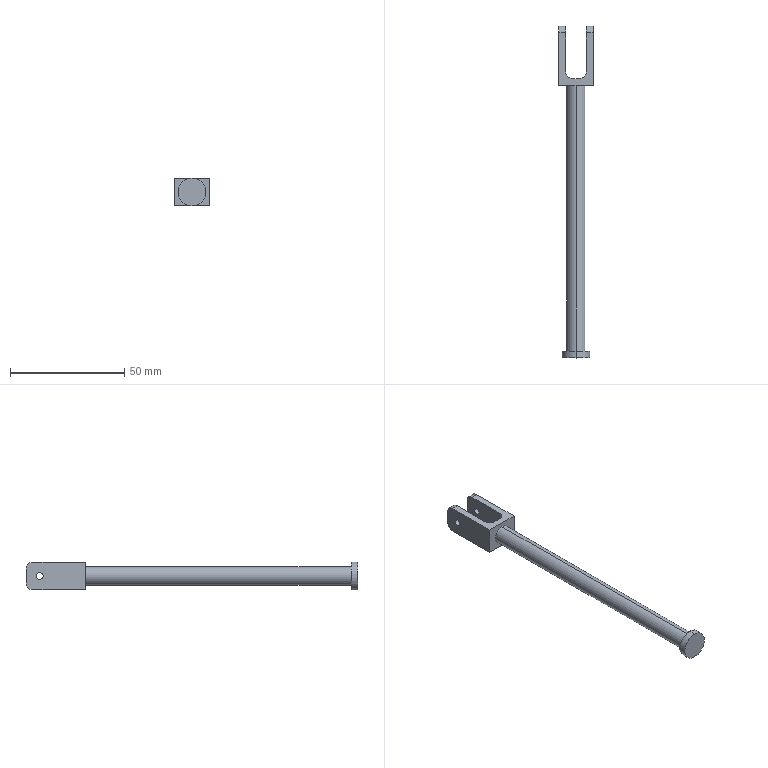Part | SolidWorks | features ICE 3, Fillet 2, Extrusion 1 | 1 solid | 26 faces | box 15 x 145 x 12.163 mm | volume 8356 mm3 | cylinder 14 | plane 12 | commonest cylinder face diameters 6 x6 3 x4 8 x2 12.163 x2
STEP:
#1=CARTESIAN_POINT('',(7.5,-119.,-0.08166));
#2=VERTEX_POINT('',#1);
#3=CARTESIAN_POINT('',(7.5,-119.,12.082));
#4=VERTEX_POINT('',#3);
#5=CARTESIAN_POINT('',(7.5,-119.,6.));
#6=DIRECTION('',(0.,-1.,0.));
#7=DIRECTION('',(0.,0.,-1.));
#8=AXIS2_PLACEMENT_3D('',#5,#6,#7);
#9=CIRCLE('',#8,6.082);
#10=EDGE_CURVE('',#2,#4,#9,.T.);
#11=ORIENTED_EDGE('',*,*,#10,.F.);
#12=CARTESIAN_POINT('',(7.5,-116.,-0.08166));
#13=VERTEX_POINT('',#12);
#14=CARTESIAN_POINT('',(7.5,-119.,-0.08166));
#15=DIRECTION('',(0.,1.,0.));
#16=VECTOR('',#15,1000.);
#17=LINE('',#14,#16);
#18=EDGE_CURVE('',#2,#13,#17,.T.);
#19=ORIENTED_EDGE('',*,*,#18,.T.);
#20=CARTESIAN_POINT('',(7.5,-116.,12.082));
#21=VERTEX_POINT('',#20);
#22=CARTESIAN_POINT('',(7.5,-116.,6.));
#23=DIRECTION('',(0.,-1.,0.));
#24=DIRECTION('',(0.,0.,-1.));
#25=AXIS2_PLACEMENT_3D('',#22,#23,#24);
#26=CIRCLE('',#25,6.082);
#27=EDGE_CURVE('',#13,#21,#26,.T.);
#28=ORIENTED_EDGE('',*,*,#27,.T.);
#29=CARTESIAN_POINT('',(7.5,-119.,12.082));
#30=DIRECTION('',(0.,1.,0.));
#31=VECTOR('',#30,1000.);
#32=LINE('',#29,#31);
#33=EDGE_CURVE('',#4,#21,#32,.T.);
#34=ORIENTED_EDGE('',*,*,#33,.F.);
#35=EDGE_LOOP('',(#11,#19,#28,#34));
#36=FACE_OUTER_BOUND('',#35,.T.);
#37=CARTESIAN_POINT('',(7.5,-119.,6.));
#38=DIRECTION('',(0.,1.,0.));
#39=DIRECTION('',(0.,0.,1.));
#40=AXIS2_PLACEMENT_3D('',#37,#38,#39);
#41=CYLINDRICAL_SURFACE('',#40,6.082);
#42=ADVANCED_FACE('',(#36),#41,.T.);
#43=CARTESIAN_POINT('',(7.5,-116.,2.));
#44=VERTEX_POINT('',#43);
#45=CARTESIAN_POINT('',(7.5,-116.,10.));
#46=VERTEX_POINT('',#45);
#47=CARTESIAN_POINT('',(7.5,-116.,6.));
#48=DIRECTION('',(0.,-1.,0.));
#49=DIRECTION('',(0.,0.,-1.));
#50=AXIS2_PLACEMENT_3D('',#47,#48,#49);
#51=CIRCLE('',#50,4.);
#52=EDGE_CURVE('',#44,#46,#51,.T.);
#53=ORIENTED_EDGE('',*,*,#52,.F.);
#54=CARTESIAN_POINT('',(7.5,0.,2.));
#55=VERTEX_POINT('',#54);
#56=CARTESIAN_POINT('',(7.5,-116.,2.));
#57=DIRECTION('',(0.,1.,0.));
#58=VECTOR('',#57,1000.);
#59=LINE('',#56,#58);
#60=EDGE_CURVE('',#44,#55,#59,.T.);
#61=ORIENTED_EDGE('',*,*,#60,.T.);
#62=CARTESIAN_POINT('',(7.5,0.,10.));
#63=VERTEX_POINT('',#62);
#64=CARTESIAN_POINT('',(7.5,0.,6.));
#65=DIRECTION('',(0.,-1.,0.));
#66=DIRECTION('',(0.,0.,-1.));
#67=AXIS2_PLACEMENT_3D('',#64,#65,#66);
#68=CIRCLE('',#67,4.);
#69=EDGE_CURVE('',#55,#63,#68,.T.);
#70=ORIENTED_EDGE('',*,*,#69,.T.);
#71=CARTESIAN_POINT('',(7.5,-116.,10.));
#72=DIRECTION('',(0.,1.,0.));
#73=VECTOR('',#72,1000.);
#74=LINE('',#71,#73);
#75=EDGE_CURVE('',#46,#63,#74,.T.);
#76=ORIENTED_EDGE('',*,*,#75,.F.);
#77=EDGE_LOOP('',(#53,#61,#70,#76));
#78=FACE_OUTER_BOUND('',#77,.T.);
#79=CARTESIAN_POINT('',(7.5,-116.,6.));
#80=DIRECTION('',(0.,1.,0.));
#81=DIRECTION('',(0.,0.,1.));
#82=AXIS2_PLACEMENT_3D('',#79,#80,#81);
#83=CYLINDRICAL_SURFACE('',#82,4.);
#84=ADVANCED_FACE('',(#78),#83,.T.);
#85=CARTESIAN_POINT('',(12.,18.5,6.));
#86=VERTEX_POINT('',#85);
#87=CARTESIAN_POINT('',(12.,21.5,6.));
#88=VERTEX_POINT('',#87);
#89=CARTESIAN_POINT('',(12.,20.,6.));
#90=DIRECTION('',(1.,0.,0.));
#91=DIRECTION('',(0.,0.,-1.));
#92=AXIS2_PLACEMENT_3D('',#89,#90,#91);
#93=CIRCLE('',#92,1.5);
#94=EDGE_CURVE('',#86,#88,#93,.T.);
#95=ORIENTED_EDGE('',*,*,#94,.F.);
#96=CARTESIAN_POINT('',(15.,18.5,6.));
#97=VERTEX_POINT('',#96);
#98=CARTESIAN_POINT('',(0.,18.5,6.));
#99=DIRECTION('',(1.,0.,0.));
#100=VECTOR('',#99,1000.);
#101=LINE('',#98,#100);
#102=EDGE_CURVE('',#86,#97,#101,.T.);
#103=ORIENTED_EDGE('',*,*,#102,.T.);
#104=CARTESIAN_POINT('',(15.,21.5,6.));
#105=VERTEX_POINT('',#104);
#106=CARTESIAN_POINT('',(15.,20.,6.));
#107=DIRECTION('',(1.,0.,0.));
#108=DIRECTION('',(0.,1.,0.));
#109=AXIS2_PLACEMENT_3D('',#106,#107,#108);
#110=CIRCLE('',#109,1.5);
#111=EDGE_CURVE('',#97,#105,#110,.T.);
#112=ORIENTED_EDGE('',*,*,#111,.T.);
#113=CARTESIAN_POINT('',(0.,21.5,6.));
#114=DIRECTION('',(1.,0.,0.));
#115=VECTOR('',#114,1000.);
#116=LINE('',#113,#115);
#117=EDGE_CURVE('',#88,#105,#116,.T.);
#118=ORIENTED_EDGE('',*,*,#117,.F.);
#119=EDGE_LOOP('',(#95,#103,#112,#118));
#120=FACE_OUTER_BOUND('',#119,.T.);
#121=CARTESIAN_POINT('',(0.,20.,6.));
#122=DIRECTION('',(1.,0.,0.));
#123=DIRECTION('',(0.,1.,0.));
#124=AXIS2_PLACEMENT_3D('',#121,#122,#123);
#125=CYLINDRICAL_SURFACE('',#124,1.5);
#126=ADVANCED_FACE('',(#120),#125,.F.);
#127=CARTESIAN_POINT('',(0.,18.5,6.));
#128=VERTEX_POINT('',#127);
#129=CARTESIAN_POINT('',(0.,21.5,6.));
#130=VERTEX_POINT('',#129);
#131=CARTESIAN_POINT('',(0.,20.,6.));
#132=DIRECTION('',(1.,0.,0.));
#133=DIRECTION('',(0.,1.,0.));
#134=AXIS2_PLACEMENT_3D('',#131,#132,#133);
#135=CIRCLE('',#134,1.5);
#136=EDGE_CURVE('',#128,#130,#135,.T.);
#137=ORIENTED_EDGE('',*,*,#136,.F.);
#138=CARTESIAN_POINT('',(3.,18.5,6.));
#139=VERTEX_POINT('',#138);
#140=CARTESIAN_POINT('',(0.,18.5,6.));
#141=DIRECTION('',(1.,0.,0.));
#142=VECTOR('',#141,1000.);
#143=LINE('',#140,#142);
#144=EDGE_CURVE('',#128,#139,#143,.T.);
#145=ORIENTED_EDGE('',*,*,#144,.T.);
#146=CARTESIAN_POINT('',(3.,21.5,6.));
#147=VERTEX_POINT('',#146);
#148=CARTESIAN_POINT('',(3.,20.,6.));
#149=DIRECTION('',(-1.,0.,0.));
#150=DIRECTION('',(0.,0.,1.));
#151=AXIS2_PLACEMENT_3D('',#148,#149,#150);
#152=CIRCLE('',#151,1.5);
#153=EDGE_CURVE('',#147,#139,#152,.T.);
#154=ORIENTED_EDGE('',*,*,#153,.F.);
#155=CARTESIAN_POINT('',(0.,21.5,6.));
#156=DIRECTION('',(1.,0.,0.));
#157=VECTOR('',#156,1000.);
#158=LINE('',#155,#157);
#159=EDGE_CURVE('',#130,#147,#158,.T.);
#160=ORIENTED_EDGE('',*,*,#159,.F.);
#161=EDGE_LOOP('',(#137,#145,#154,#160));
#162=FACE_OUTER_BOUND('',#161,.T.);
#163=CARTESIAN_POINT('',(0.,20.,6.));
#164=DIRECTION('',(1.,0.,0.));
#165=DIRECTION('',(0.,1.,0.));
#166=AXIS2_PLACEMENT_3D('',#163,#164,#165);
#167=CYLINDRICAL_SURFACE('',#166,1.5);
#168=ADVANCED_FACE('',(#162),#167,.F.);
#169=CARTESIAN_POINT('',(3.,26.,9.));
#170=VERTEX_POINT('',#169);
#171=CARTESIAN_POINT('',(3.,26.,3.));
#172=VERTEX_POINT('',#171);
#173=CARTESIAN_POINT('',(3.,26.,12.));
#174=DIRECTION('',(0.,0.,-1.));
#175=VECTOR('',#174,1000.);
#176=LINE('',#173,#175);
#177=EDGE_CURVE('',#170,#172,#176,.T.);
#178=ORIENTED_EDGE('',*,*,#177,.T.);
#179=CARTESIAN_POINT('',(0.,26.,3.));
#180=VERTEX_POINT('',#179);
#181=CARTESIAN_POINT('',(3.,26.,3.));
#182=DIRECTION('',(-1.,0.,0.));
#183=VECTOR('',#182,1000.);
#184=LINE('',#181,#183);
#185=EDGE_CURVE('',#172,#180,#184,.T.);
#186=ORIENTED_EDGE('',*,*,#185,.T.);
#187=CARTESIAN_POINT('',(0.,26.,9.));
#188=VERTEX_POINT('',#187);
#189=CARTESIAN_POINT('',(0.,26.,12.));
#190=DIRECTION('',(0.,0.,-1.));
#191=VECTOR('',#190,1000.);
#192=LINE('',#189,#191);
#193=EDGE_CURVE('',#188,#180,#192,.T.);
#194=ORIENTED_EDGE('',*,*,#193,.F.);
#195=CARTESIAN_POINT('',(3.,26.,9.));
#196=DIRECTION('',(1.,0.,0.));
#197=VECTOR('',#196,1000.);
#198=LINE('',#195,#197);
#199=EDGE_CURVE('',#188,#170,#198,.T.);
#200=ORIENTED_EDGE('',*,*,#199,.T.);
#201=EDGE_LOOP('',(#178,#186,#194,#200));
#202=FACE_OUTER_BOUND('',#201,.T.);
#203=CARTESIAN_POINT('',(3.,26.,12.));
#204=DIRECTION('',(0.,-1.,0.));
#205=DIRECTION('',(0.,0.,-1.));
#206=AXIS2_PLACEMENT_3D('',#203,#204,#205);
#207=PLANE('',#206);
#208=ADVANCED_FACE('',(#202),#207,.F.);
#209=CARTESIAN_POINT('',(0.,20.,6.));
#210=DIRECTION('',(1.,0.,0.));
#211=DIRECTION('',(0.,1.,0.));
#212=AXIS2_PLACEMENT_3D('',#209,#210,#211);
#213=CIRCLE('',#212,1.5);
#214=EDGE_CURVE('',#130,#128,#213,.T.);
#215=ORIENTED_EDGE('',*,*,#214,.T.);
#216=ORIENTED_EDGE('',*,*,#136,.T.);
#217=EDGE_LOOP('',(#215,#216));
#218=FACE_BOUND('',#217,.T.);
#219=ORIENTED_EDGE('',*,*,#193,.T.);
#220=CARTESIAN_POINT('',(0.,23.,0.));
#221=VERTEX_POINT('',#220);
#222=CARTESIAN_POINT('',(0.,23.,3.));
#223=DIRECTION('',(-1.,0.,0.));
#224=DIRECTION('',(0.,1.,0.));
#225=AXIS2_PLACEMENT_3D('',#222,#223,#224);
#226=CIRCLE('',#225,3.);
#227=EDGE_CURVE('',#180,#221,#226,.T.);
#228=ORIENTED_EDGE('',*,*,#227,.T.);
#229=CARTESIAN_POINT('',(0.,0.,0.));
#230=VERTEX_POINT('',#229);
#231=CARTESIAN_POINT('',(0.,26.,0.));
#232=DIRECTION('',(0.,-1.,0.));
#233=VECTOR('',#232,1000.);
#234=LINE('',#231,#233);
#235=EDGE_CURVE('',#221,#230,#234,.T.);
#236=ORIENTED_EDGE('',*,*,#235,.T.);
#237=CARTESIAN_POINT('',(0.,0.,12.));
#238=VERTEX_POINT('',#237);
#239=CARTESIAN_POINT('',(0.,0.,12.));
#240=DIRECTION('',(0.,0.,-1.));
#241=VECTOR('',#240,1000.);
#242=LINE('',#239,#241);
#243=EDGE_CURVE('',#238,#230,#242,.T.);
#244=ORIENTED_EDGE('',*,*,#243,.F.);
#245=CARTESIAN_POINT('',(0.,23.,12.));
#246=VERTEX_POINT('',#245);
#247=CARTESIAN_POINT('',(0.,26.,12.));
#248=DIRECTION('',(0.,-1.,0.));
#249=VECTOR('',#248,1000.);
#250=LINE('',#247,#249);
#251=EDGE_CURVE('',#246,#238,#250,.T.);
#252=ORIENTED_EDGE('',*,*,#251,.F.);
#253=CARTESIAN_POINT('',(0.,23.,9.));
#254=DIRECTION('',(-1.,0.,0.));
#255=DIRECTION('',(0.,1.,0.));
#256=AXIS2_PLACEMENT_3D('',#253,#254,#255);
#257=CIRCLE('',#256,3.);
#258=EDGE_CURVE('',#246,#188,#257,.T.);
#259=ORIENTED_EDGE('',*,*,#258,.T.);
#260=EDGE_LOOP('',(#219,#228,#236,#244,#252,#259));
#261=FACE_OUTER_BOUND('',#260,.T.);
#262=CARTESIAN_POINT('',(0.,26.,12.));
#263=DIRECTION('',(1.,0.,0.));
#264=DIRECTION('',(0.,1.,0.));
#265=AXIS2_PLACEMENT_3D('',#262,#263,#264);
#266=PLANE('',#265);
#267=ADVANCED_FACE('',(#218,#261),#266,.F.);
#268=CARTESIAN_POINT('',(7.5,0.,6.));
#269=DIRECTION('',(0.,-1.,0.));
#270=DIRECTION('',(0.,0.,-1.));
#271=AXIS2_PLACEMENT_3D('',#268,#269,#270);
#272=CIRCLE('',#271,4.);
#273=EDGE_CURVE('',#63,#55,#272,.T.);
#274=ORIENTED_EDGE('',*,*,#273,.F.);
#275=ORIENTED_EDGE('',*,*,#69,.F.);
#276=EDGE_LOOP('',(#274,#275));
#277=FACE_BOUND('',#276,.T.);
#278=CARTESIAN_POINT('',(15.,0.,0.));
#279=VERTEX_POINT('',#278);
#280=CARTESIAN_POINT('',(0.,0.,0.));
#281=DIRECTION('',(1.,0.,0.));
#282=VECTOR('',#281,1000.);
#283=LINE('',#280,#282);
#284=EDGE_CURVE('',#230,#279,#283,.T.);
#285=ORIENTED_EDGE('',*,*,#284,.T.);
#286=CARTESIAN_POINT('',(15.,0.,12.));
#287=VERTEX_POINT('',#286);
#288=CARTESIAN_POINT('',(15.,0.,12.));
#289=DIRECTION('',(0.,0.,-1.));
#290=VECTOR('',#289,1000.);
#291=LINE('',#288,#290);
#292=EDGE_CURVE('',#287,#279,#291,.T.);
#293=ORIENTED_EDGE('',*,*,#292,.F.);
#294=CARTESIAN_POINT('',(0.,0.,12.));
#295=DIRECTION('',(1.,0.,0.));
#296=VECTOR('',#295,1000.);
#297=LINE('',#294,#296);
#298=EDGE_CURVE('',#238,#287,#297,.T.);
#299=ORIENTED_EDGE('',*,*,#298,.F.);
#300=ORIENTED_EDGE('',*,*,#243,.T.);
#301=EDGE_LOOP('',(#285,#293,#299,#300));
#302=FACE_OUTER_BOUND('',#301,.T.);
#303=CARTESIAN_POINT('',(0.,0.,12.));
#304=DIRECTION('',(0.,1.,0.));
#305=DIRECTION('',(0.,0.,1.));
#306=AXIS2_PLACEMENT_3D('',#303,#304,#305);
#307=PLANE('',#306);
#308=ADVANCED_FACE('',(#277,#302),#307,.F.);
#309=CARTESIAN_POINT('',(15.,20.,6.));
#310=DIRECTION('',(1.,0.,0.));
#311=DIRECTION('',(0.,1.,0.));
#312=AXIS2_PLACEMENT_3D('',#309,#310,#311);
#313=CIRCLE('',#312,1.5);
#314=EDGE_CURVE('',#105,#97,#313,.T.);
#315=ORIENTED_EDGE('',*,*,#314,.F.);
#316=ORIENTED_EDGE('',*,*,#111,.F.);
#317=EDGE_LOOP('',(#315,#316));
#318=FACE_BOUND('',#317,.T.);
#319=CARTESIAN_POINT('',(15.,23.,0.));
#320=VERTEX_POINT('',#319);
#321=CARTESIAN_POINT('',(15.,0.,0.));
#322=DIRECTION('',(0.,1.,0.));
#323=VECTOR('',#322,1000.);
#324=LINE('',#321,#323);
#325=EDGE_CURVE('',#279,#320,#324,.T.);
#326=ORIENTED_EDGE('',*,*,#325,.T.);
#327=CARTESIAN_POINT('',(15.,26.,3.));
#328=VERTEX_POINT('',#327);
#329=CARTESIAN_POINT('',(15.,23.,3.));
#330=DIRECTION('',(1.,0.,0.));
#331=DIRECTION('',(0.,-1.,0.));
#332=AXIS2_PLACEMENT_3D('',#329,#330,#331);
#333=CIRCLE('',#332,3.);
#334=EDGE_CURVE('',#320,#328,#333,.T.);
#335=ORIENTED_EDGE('',*,*,#334,.T.);
#336=CARTESIAN_POINT('',(15.,26.,9.));
#337=VERTEX_POINT('',#336);
#338=CARTESIAN_POINT('',(15.,26.,12.));
#339=DIRECTION('',(0.,0.,-1.));
#340=VECTOR('',#339,1000.);
#341=LINE('',#338,#340);
#342=EDGE_CURVE('',#337,#328,#341,.T.);
#343=ORIENTED_EDGE('',*,*,#342,.F.);
#344=CARTESIAN_POINT('',(15.,23.,12.));
#345=VERTEX_POINT('',#344);
#346=CARTESIAN_POINT('',(15.,23.,9.));
#347=DIRECTION('',(1.,0.,0.));
#348=DIRECTION('',(0.,-1.,0.));
#349=AXIS2_PLACEMENT_3D('',#346,#347,#348);
#350=CIRCLE('',#349,3.);
#351=EDGE_CURVE('',#337,#345,#350,.T.);
#352=ORIENTED_EDGE('',*,*,#351,.T.);
#353=CARTESIAN_POINT('',(15.,0.,12.));
#354=DIRECTION('',(0.,1.,0.));
#355=VECTOR('',#354,1000.);
#356=LINE('',#353,#355);
#357=EDGE_CURVE('',#287,#345,#356,.T.);
#358=ORIENTED_EDGE('',*,*,#357,.F.);
#359=ORIENTED_EDGE('',*,*,#292,.T.);
#360=EDGE_LOOP('',(#326,#335,#343,#352,#358,#359));
#361=FACE_OUTER_BOUND('',#360,.T.);
#362=CARTESIAN_POINT('',(15.,0.,12.));
#363=DIRECTION('',(-1.,0.,0.));
#364=DIRECTION('',(0.,-1.,0.));
#365=AXIS2_PLACEMENT_3D('',#362,#363,#364);
#366=PLANE('',#365);
#367=ADVANCED_FACE('',(#318,#361),#366,.F.);
#368=ORIENTED_EDGE('',*,*,#342,.T.);
#369=CARTESIAN_POINT('',(12.,26.,3.));
#370=VERTEX_POINT('',#369);
#371=CARTESIAN_POINT('',(15.,26.,3.));
#372=DIRECTION('',(-1.,0.,0.));
#373=VECTOR('',#372,1000.);
#374=LINE('',#371,#373);
#375=EDGE_CURVE('',#328,#370,#374,.T.);
#376=ORIENTED_EDGE('',*,*,#375,.T.);
#377=CARTESIAN_POINT('',(12.,26.,9.));
#378=VERTEX_POINT('',#377);
#379=CARTESIAN_POINT('',(12.,26.,12.));
#380=DIRECTION('',(0.,0.,-1.));
#381=VECTOR('',#380,1000.);
#382=LINE('',#379,#381);
#383=EDGE_CURVE('',#378,#370,#382,.T.);
#384=ORIENTED_EDGE('',*,*,#383,.F.);
#385=CARTESIAN_POINT('',(15.,26.,9.));
#386=DIRECTION('',(1.,0.,0.));
#387=VECTOR('',#386,1000.);
#388=LINE('',#385,#387);
#389=EDGE_CURVE('',#378,#337,#388,.T.);
#390=ORIENTED_EDGE('',*,*,#389,.T.);
#391=EDGE_LOOP('',(#368,#376,#384,#390));
#392=FACE_OUTER_BOUND('',#391,.T.);
#393=CARTESIAN_POINT('',(15.,26.,12.));
#394=DIRECTION('',(0.,-1.,0.));
#395=DIRECTION('',(0.,0.,-1.));
#396=AXIS2_PLACEMENT_3D('',#393,#394,#395);
#397=PLANE('',#396);
#398=ADVANCED_FACE('',(#392),#397,.F.);
#399=CARTESIAN_POINT('',(12.,20.,6.));
#400=DIRECTION('',(1.,0.,0.));
#401=DIRECTION('',(0.,0.,-1.));
#402=AXIS2_PLACEMENT_3D('',#399,#400,#401);
#403=CIRCLE('',#402,1.5);
#404=EDGE_CURVE('',#88,#86,#403,.T.);
#405=ORIENTED_EDGE('',*,*,#404,.T.);
#406=ORIENTED_EDGE('',*,*,#94,.T.);
#407=EDGE_LOOP('',(#405,#406));
#408=FACE_BOUND('',#407,.T.);
#409=CARTESIAN_POINT('',(12.,23.,0.));
#410=VERTEX_POINT('',#409);
#411=CARTESIAN_POINT('',(12.,6.,0.));
#412=VERTEX_POINT('',#411);
#413=CARTESIAN_POINT('',(12.,26.,0.));
#414=DIRECTION('',(0.,-1.,0.));
#415=VECTOR('',#414,1000.);
#416=LINE('',#413,#415);
#417=EDGE_CURVE('',#410,#412,#416,.T.);
#418=ORIENTED_EDGE('',*,*,#417,.T.);
#419=CARTESIAN_POINT('',(12.,6.,12.));
#420=VERTEX_POINT('',#419);
#421=CARTESIAN_POINT('',(12.,6.,12.));
#422=DIRECTION('',(0.,0.,1.));
#423=VECTOR('',#422,1000.);
#424=LINE('',#421,#423);
#425=EDGE_CURVE('',#412,#420,#424,.T.);
#426=ORIENTED_EDGE('',*,*,#425,.T.);
#427=CARTESIAN_POINT('',(12.,23.,12.));
#428=VERTEX_POINT('',#427);
#429=CARTESIAN_POINT('',(12.,26.,12.));
#430=DIRECTION('',(0.,-1.,0.));
#431=VECTOR('',#430,1000.);
#432=LINE('',#429,#431);
#433=EDGE_CURVE('',#428,#420,#432,.T.);
#434=ORIENTED_EDGE('',*,*,#433,.F.);
#435=CARTESIAN_POINT('',(12.,23.,9.));
#436=DIRECTION('',(-1.,0.,0.));
#437=DIRECTION('',(0.,0.,-1.));
#438=AXIS2_PLACEMENT_3D('',#435,#436,#437);
#439=CIRCLE('',#438,3.);
#440=EDGE_CURVE('',#428,#378,#439,.T.);
#441=ORIENTED_EDGE('',*,*,#440,.T.);
#442=ORIENTED_EDGE('',*,*,#383,.T.);
#443=CARTESIAN_POINT('',(12.,23.,3.));
#444=DIRECTION('',(-1.,0.,0.));
#445=DIRECTION('',(0.,0.,-1.));
#446=AXIS2_PLACEMENT_3D('',#443,#444,#445);
#447=CIRCLE('',#446,3.);
#448=EDGE_CURVE('',#370,#410,#447,.T.);
#449=ORIENTED_EDGE('',*,*,#448,.T.);
#450=EDGE_LOOP('',(#418,#426,#434,#441,#442,#449));
#451=FACE_OUTER_BOUND('',#450,.T.);
#452=CARTESIAN_POINT('',(12.,26.,12.));
#453=DIRECTION('',(1.,0.,0.));
#454=DIRECTION('',(0.,0.,-1.));
#455=AXIS2_PLACEMENT_3D('',#452,#453,#454);
#456=PLANE('',#455);
#457=ADVANCED_FACE('',(#408,#451),#456,.F.);
#458=CARTESIAN_POINT('',(9.,3.,12.));
#459=VERTEX_POINT('',#458);
#460=CARTESIAN_POINT('',(6.,3.,12.));
#461=VERTEX_POINT('',#460);
#462=CARTESIAN_POINT('',(12.,3.,12.));
#463=DIRECTION('',(-1.,0.,0.));
#464=VECTOR('',#463,1000.);
#465=LINE('',#462,#464);
#466=EDGE_CURVE('',#459,#461,#465,.T.);
#467=ORIENTED_EDGE('',*,*,#466,.F.);
#468=CARTESIAN_POINT('',(9.,3.,0.));
#469=VERTEX_POINT('',#468);
#470=CARTESIAN_POINT('',(9.,3.,0.));
#471=DIRECTION('',(0.,0.,-1.));
#472=VECTOR('',#471,1000.);
#473=LINE('',#470,#472);
#474=EDGE_CURVE('',#459,#469,#473,.T.);
#475=ORIENTED_EDGE('',*,*,#474,.T.);
#476=CARTESIAN_POINT('',(6.,3.,0.));
#477=VERTEX_POINT('',#476);
#478=CARTESIAN_POINT('',(12.,3.,0.));
#479=DIRECTION('',(-1.,0.,0.));
#480=VECTOR('',#479,1000.);
#481=LINE('',#478,#480);
#482=EDGE_CURVE('',#469,#477,#481,.T.);
#483=ORIENTED_EDGE('',*,*,#482,.T.);
#484=CARTESIAN_POINT('',(6.,3.,12.));
#485=DIRECTION('',(0.,0.,1.));
#486=VECTOR('',#485,1000.);
#487=LINE('',#484,#486);
#488=EDGE_CURVE('',#477,#461,#487,.T.);
#489=ORIENTED_EDGE('',*,*,#488,.T.);
#490=EDGE_LOOP('',(#467,#475,#483,#489));
#491=FACE_OUTER_BOUND('',#490,.T.);
#492=CARTESIAN_POINT('',(12.,3.,12.));
#493=DIRECTION('',(0.,-1.,0.));
#494=DIRECTION('',(1.,0.,0.));
#495=AXIS2_PLACEMENT_3D('',#492,#493,#494);
#496=PLANE('',#495);
#497=ADVANCED_FACE('',(#491),#496,.F.);
#498=ORIENTED_EDGE('',*,*,#153,.T.);
#499=CARTESIAN_POINT('',(3.,20.,6.));
#500=DIRECTION('',(-1.,0.,0.));
#501=DIRECTION('',(0.,0.,1.));
#502=AXIS2_PLACEMENT_3D('',#499,#500,#501);
#503=CIRCLE('',#502,1.5);
#504=EDGE_CURVE('',#139,#147,#503,.T.);
#505=ORIENTED_EDGE('',*,*,#504,.T.);
#506=EDGE_LOOP('',(#498,#505));
#507=FACE_BOUND('',#506,.T.);
#508=CARTESIAN_POINT('',(3.,6.,12.));
#509=VERTEX_POINT('',#508);
#510=CARTESIAN_POINT('',(3.,23.,12.));
#511=VERTEX_POINT('',#510);
#512=CARTESIAN_POINT('',(3.,3.,12.));
#513=DIRECTION('',(0.,1.,0.));
#514=VECTOR('',#513,1000.);
#515=LINE('',#512,#514);
#516=EDGE_CURVE('',#509,#511,#515,.T.);
#517=ORIENTED_EDGE('',*,*,#516,.F.);
#518=CARTESIAN_POINT('',(3.,6.,0.));
#519=VERTEX_POINT('',#518);
#520=CARTESIAN_POINT('',(3.,6.,0.));
#521=DIRECTION('',(0.,0.,-1.));
#522=VECTOR('',#521,1000.);
#523=LINE('',#520,#522);
#524=EDGE_CURVE('',#509,#519,#523,.T.);
#525=ORIENTED_EDGE('',*,*,#524,.T.);
#526=CARTESIAN_POINT('',(3.,23.,0.));
#527=VERTEX_POINT('',#526);
#528=CARTESIAN_POINT('',(3.,3.,0.));
#529=DIRECTION('',(0.,1.,0.));
#530=VECTOR('',#529,1000.);
#531=LINE('',#528,#530);
#532=EDGE_CURVE('',#519,#527,#531,.T.);
#533=ORIENTED_EDGE('',*,*,#532,.T.);
#534=CARTESIAN_POINT('',(3.,23.,3.));
#535=DIRECTION('',(1.,0.,0.));
#536=DIRECTION('',(0.,0.,1.));
#537=AXIS2_PLACEMENT_3D('',#534,#535,#536);
#538=CIRCLE('',#537,3.);
#539=EDGE_CURVE('',#527,#172,#538,.T.);
#540=ORIENTED_EDGE('',*,*,#539,.T.);
#541=ORIENTED_EDGE('',*,*,#177,.F.);
#542=CARTESIAN_POINT('',(3.,23.,9.));
#543=DIRECTION('',(1.,0.,0.));
#544=DIRECTION('',(0.,0.,1.));
#545=AXIS2_PLACEMENT_3D('',#542,#543,#544);
#546=CIRCLE('',#545,3.);
#547=EDGE_CURVE('',#170,#511,#546,.T.);
#548=ORIENTED_EDGE('',*,*,#547,.T.);
#549=EDGE_LOOP('',(#517,#525,#533,#540,#541,#548));
#550=FACE_OUTER_BOUND('',#549,.T.);
#551=CARTESIAN_POINT('',(3.,3.,12.));
#552=DIRECTION('',(-1.,0.,0.));
#553=DIRECTION('',(0.,0.,1.));
#554=AXIS2_PLACEMENT_3D('',#551,#552,#553);
#555=PLANE('',#554);
#556=ADVANCED_FACE('',(#507,#550),#555,.F.);
#557=ORIENTED_EDGE('',*,*,#357,.T.);
#558=CARTESIAN_POINT('',(12.,23.,12.));
#559=DIRECTION('',(-1.,0.,0.));
#560=VECTOR('',#559,1000.);
#561=LINE('',#558,#560);
#562=EDGE_CURVE('',#345,#428,#561,.T.);
#563=ORIENTED_EDGE('',*,*,#562,.T.);
#564=ORIENTED_EDGE('',*,*,#433,.T.);
#565=CARTESIAN_POINT('',(9.,6.,12.));
#566=DIRECTION('',(0.,0.,-1.));
#567=DIRECTION('',(1.,0.,0.));
#568=AXIS2_PLACEMENT_3D('',#565,#566,#567);
#569=CIRCLE('',#568,3.);
#570=EDGE_CURVE('',#420,#459,#569,.T.);
#571=ORIENTED_EDGE('',*,*,#570,.T.);
#572=ORIENTED_EDGE('',*,*,#466,.T.);
#573=CARTESIAN_POINT('',(6.,6.,12.));
#574=DIRECTION('',(0.,0.,-1.));
#575=DIRECTION('',(1.,0.,0.));
#576=AXIS2_PLACEMENT_3D('',#573,#574,#575);
#577=CIRCLE('',#576,3.);
#578=EDGE_CURVE('',#461,#509,#577,.T.);
#579=ORIENTED_EDGE('',*,*,#578,.T.);
#580=ORIENTED_EDGE('',*,*,#516,.T.);
#581=CARTESIAN_POINT('',(0.,23.,12.));
#582=DIRECTION('',(-1.,0.,0.));
#583=VECTOR('',#582,1000.);
#584=LINE('',#581,#583);
#585=EDGE_CURVE('',#511,#246,#584,.T.);
#586=ORIENTED_EDGE('',*,*,#585,.T.);
#587=ORIENTED_EDGE('',*,*,#251,.T.);
#588=ORIENTED_EDGE('',*,*,#298,.T.);
#589=EDGE_LOOP('',(#557,#563,#564,#571,#572,#579,#580,#586,#587,#588));
#590=FACE_OUTER_BOUND('',#589,.T.);
#591=CARTESIAN_POINT('',(0.,0.,12.));
#592=DIRECTION('',(0.,0.,1.));
#593=DIRECTION('',(1.,0.,0.));
#594=AXIS2_PLACEMENT_3D('',#591,#592,#593);
#595=PLANE('',#594);
#596=ADVANCED_FACE('',(#590),#595,.T.);
#597=ORIENTED_EDGE('',*,*,#235,.F.);
#598=CARTESIAN_POINT('',(0.,23.,0.));
#599=DIRECTION('',(1.,0.,0.));
#600=VECTOR('',#599,1000.);
#601=LINE('',#598,#600);
#602=EDGE_CURVE('',#221,#527,#601,.T.);
#603=ORIENTED_EDGE('',*,*,#602,.T.);
#604=ORIENTED_EDGE('',*,*,#532,.F.);
#605=CARTESIAN_POINT('',(6.,6.,0.));
#606=DIRECTION('',(0.,0.,1.));
#607=DIRECTION('',(1.,0.,0.));
#608=AXIS2_PLACEMENT_3D('',#605,#606,#607);
#609=CIRCLE('',#608,3.);
#610=EDGE_CURVE('',#519,#477,#609,.T.);
#611=ORIENTED_EDGE('',*,*,#610,.T.);
#612=ORIENTED_EDGE('',*,*,#482,.F.);
#613=CARTESIAN_POINT('',(9.,6.,0.));
#614=DIRECTION('',(0.,0.,1.));
#615=DIRECTION('',(1.,0.,0.));
#616=AXIS2_PLACEMENT_3D('',#613,#614,#615);
#617=CIRCLE('',#616,3.);
#618=EDGE_CURVE('',#469,#412,#617,.T.);
#619=ORIENTED_EDGE('',*,*,#618,.T.);
#620=ORIENTED_EDGE('',*,*,#417,.F.);
#621=CARTESIAN_POINT('',(0.,23.,0.));
#622=DIRECTION('',(1.,0.,0.));
#623=VECTOR('',#622,1000.);
#624=LINE('',#621,#623);
#625=EDGE_CURVE('',#410,#320,#624,.T.);
#626=ORIENTED_EDGE('',*,*,#625,.T.);
#627=ORIENTED_EDGE('',*,*,#325,.F.);
#628=ORIENTED_EDGE('',*,*,#284,.F.);
#629=EDGE_LOOP('',(#597,#603,#604,#611,#612,#619,#620,#626,#627,#628));
#630=FACE_OUTER_BOUND('',#629,.T.);
#631=CARTESIAN_POINT('',(0.,0.,0.));
#632=DIRECTION('',(0.,0.,1.));
#633=DIRECTION('',(1.,0.,0.));
#634=AXIS2_PLACEMENT_3D('',#631,#632,#633);
#635=PLANE('',#634);
#636=ADVANCED_FACE('',(#630),#635,.F.);
#637=ORIENTED_EDGE('',*,*,#539,.F.);
#638=ORIENTED_EDGE('',*,*,#602,.F.);
#639=ORIENTED_EDGE('',*,*,#227,.F.);
#640=ORIENTED_EDGE('',*,*,#185,.F.);
#641=EDGE_LOOP('',(#637,#638,#639,#640));
#642=FACE_OUTER_BOUND('',#641,.T.);
#643=CARTESIAN_POINT('',(3.,23.,3.));
#644=DIRECTION('',(-1.,0.,0.));
#645=DIRECTION('',(0.,0.,1.));
#646=AXIS2_PLACEMENT_3D('',#643,#644,#645);
#647=CYLINDRICAL_SURFACE('',#646,3.);
#648=ADVANCED_FACE('',(#642),#647,.T.);
#649=ORIENTED_EDGE('',*,*,#334,.F.);
#650=ORIENTED_EDGE('',*,*,#625,.F.);
#651=ORIENTED_EDGE('',*,*,#448,.F.);
#652=ORIENTED_EDGE('',*,*,#375,.F.);
#653=EDGE_LOOP('',(#649,#650,#651,#652));
#654=FACE_OUTER_BOUND('',#653,.T.);
#655=CARTESIAN_POINT('',(15.,23.,3.));
#656=DIRECTION('',(-1.,0.,0.));
#657=DIRECTION('',(0.,0.,1.));
#658=AXIS2_PLACEMENT_3D('',#655,#656,#657);
#659=CYLINDRICAL_SURFACE('',#658,3.);
#660=ADVANCED_FACE('',(#654),#659,.T.);
#661=ORIENTED_EDGE('',*,*,#351,.F.);
#662=ORIENTED_EDGE('',*,*,#389,.F.);
#663=ORIENTED_EDGE('',*,*,#440,.F.);
#664=ORIENTED_EDGE('',*,*,#562,.F.);
#665=EDGE_LOOP('',(#661,#662,#663,#664));
#666=FACE_OUTER_BOUND('',#665,.T.);
#667=CARTESIAN_POINT('',(0.,23.,9.));
#668=DIRECTION('',(1.,0.,0.));
#669=DIRECTION('',(0.,0.,-1.));
#670=AXIS2_PLACEMENT_3D('',#667,#668,#669);
#671=CYLINDRICAL_SURFACE('',#670,3.);
#672=ADVANCED_FACE('',(#666),#671,.T.);
#673=ORIENTED_EDGE('',*,*,#547,.F.);
#674=ORIENTED_EDGE('',*,*,#199,.F.);
#675=ORIENTED_EDGE('',*,*,#258,.F.);
#676=ORIENTED_EDGE('',*,*,#585,.F.);
#677=EDGE_LOOP('',(#673,#674,#675,#676));
#678=FACE_OUTER_BOUND('',#677,.T.);
#679=CARTESIAN_POINT('',(0.,23.,9.));
#680=DIRECTION('',(1.,0.,0.));
#681=DIRECTION('',(0.,0.,-1.));
#682=AXIS2_PLACEMENT_3D('',#679,#680,#681);
#683=CYLINDRICAL_SURFACE('',#682,3.);
#684=ADVANCED_FACE('',(#678),#683,.T.);
#685=ORIENTED_EDGE('',*,*,#570,.F.);
#686=ORIENTED_EDGE('',*,*,#425,.F.);
#687=ORIENTED_EDGE('',*,*,#618,.F.);
#688=ORIENTED_EDGE('',*,*,#474,.F.);
#689=EDGE_LOOP('',(#685,#686,#687,#688));
#690=FACE_OUTER_BOUND('',#689,.T.);
#691=CARTESIAN_POINT('',(9.,6.,12.));
#692=DIRECTION('',(0.,0.,1.));
#693=DIRECTION('',(1.,0.,0.));
#694=AXIS2_PLACEMENT_3D('',#691,#692,#693);
#695=CYLINDRICAL_SURFACE('',#694,3.);
#696=ADVANCED_FACE('',(#690),#695,.F.);
#697=ORIENTED_EDGE('',*,*,#578,.F.);
#698=ORIENTED_EDGE('',*,*,#488,.F.);
#699=ORIENTED_EDGE('',*,*,#610,.F.);
#700=ORIENTED_EDGE('',*,*,#524,.F.);
#701=EDGE_LOOP('',(#697,#698,#699,#700));
#702=FACE_OUTER_BOUND('',#701,.T.);
#703=CARTESIAN_POINT('',(6.,6.,12.));
#704=DIRECTION('',(0.,0.,1.));
#705=DIRECTION('',(1.,0.,0.));
#706=AXIS2_PLACEMENT_3D('',#703,#704,#705);
#707=CYLINDRICAL_SURFACE('',#706,3.);
#708=ADVANCED_FACE('',(#702),#707,.F.);
#709=ORIENTED_EDGE('',*,*,#144,.F.);
#710=ORIENTED_EDGE('',*,*,#214,.F.);
#711=ORIENTED_EDGE('',*,*,#159,.T.);
#712=ORIENTED_EDGE('',*,*,#504,.F.);
#713=EDGE_LOOP('',(#709,#710,#711,#712));
#714=FACE_OUTER_BOUND('',#713,.T.);
#715=CARTESIAN_POINT('',(0.,20.,6.));
#716=DIRECTION('',(1.,0.,0.));
#717=DIRECTION('',(0.,1.,0.));
#718=AXIS2_PLACEMENT_3D('',#715,#716,#717);
#719=CYLINDRICAL_SURFACE('',#718,1.5);
#720=ADVANCED_FACE('',(#714),#719,.F.);
#721=ORIENTED_EDGE('',*,*,#102,.F.);
#722=ORIENTED_EDGE('',*,*,#404,.F.);
#723=ORIENTED_EDGE('',*,*,#117,.T.);
#724=ORIENTED_EDGE('',*,*,#314,.T.);
#725=EDGE_LOOP('',(#721,#722,#723,#724));
#726=FACE_OUTER_BOUND('',#725,.T.);
#727=CARTESIAN_POINT('',(0.,20.,6.));
#728=DIRECTION('',(1.,0.,0.));
#729=DIRECTION('',(0.,1.,0.));
#730=AXIS2_PLACEMENT_3D('',#727,#728,#729);
#731=CYLINDRICAL_SURFACE('',#730,1.5);
#732=ADVANCED_FACE('',(#726),#731,.F.);
#733=ORIENTED_EDGE('',*,*,#60,.F.);
#734=CARTESIAN_POINT('',(7.5,-116.,6.));
#735=DIRECTION('',(0.,-1.,0.));
#736=DIRECTION('',(0.,0.,-1.));
#737=AXIS2_PLACEMENT_3D('',#734,#735,#736);
#738=CIRCLE('',#737,4.);
#739=EDGE_CURVE('',#46,#44,#738,.T.);
#740=ORIENTED_EDGE('',*,*,#739,.F.);
#741=ORIENTED_EDGE('',*,*,#75,.T.);
#742=ORIENTED_EDGE('',*,*,#273,.T.);
#743=EDGE_LOOP('',(#733,#740,#741,#742));
#744=FACE_OUTER_BOUND('',#743,.T.);
#745=CARTESIAN_POINT('',(7.5,-116.,6.));
#746=DIRECTION('',(0.,1.,0.));
#747=DIRECTION('',(0.,0.,1.));
#748=AXIS2_PLACEMENT_3D('',#745,#746,#747);
#749=CYLINDRICAL_SURFACE('',#748,4.);
#750=ADVANCED_FACE('',(#744),#749,.T.);
#751=ORIENTED_EDGE('',*,*,#18,.F.);
#752=CARTESIAN_POINT('',(7.5,-119.,6.));
#753=DIRECTION('',(0.,-1.,0.));
#754=DIRECTION('',(0.,0.,-1.));
#755=AXIS2_PLACEMENT_3D('',#752,#753,#754);
#756=CIRCLE('',#755,6.082);
#757=EDGE_CURVE('',#4,#2,#756,.T.);
#758=ORIENTED_EDGE('',*,*,#757,.F.);
#759=ORIENTED_EDGE('',*,*,#33,.T.);
#760=CARTESIAN_POINT('',(7.5,-116.,6.));
#761=DIRECTION('',(0.,-1.,0.));
#762=DIRECTION('',(0.,0.,-1.));
#763=AXIS2_PLACEMENT_3D('',#760,#761,#762);
#764=CIRCLE('',#763,6.082);
#765=EDGE_CURVE('',#21,#13,#764,.T.);
#766=ORIENTED_EDGE('',*,*,#765,.T.);
#767=EDGE_LOOP('',(#751,#758,#759,#766));
#768=FACE_OUTER_BOUND('',#767,.T.);
#769=CARTESIAN_POINT('',(7.5,-119.,6.));
#770=DIRECTION('',(0.,1.,0.));
#771=DIRECTION('',(0.,0.,1.));
#772=AXIS2_PLACEMENT_3D('',#769,#770,#771);
#773=CYLINDRICAL_SURFACE('',#772,6.082);
#774=ADVANCED_FACE('',(#768),#773,.T.);
#775=ORIENTED_EDGE('',*,*,#757,.T.);
#776=ORIENTED_EDGE('',*,*,#10,.T.);
#777=EDGE_LOOP('',(#775,#776));
#778=FACE_OUTER_BOUND('',#777,.T.);
#779=CARTESIAN_POINT('',(7.5,-119.,6.));
#780=DIRECTION('',(0.,-1.,0.));
#781=DIRECTION('',(0.,0.,-1.));
#782=AXIS2_PLACEMENT_3D('',#779,#780,#781);
#783=PLANE('',#782);
#784=ADVANCED_FACE('',(#778),#783,.T.);
#785=ORIENTED_EDGE('',*,*,#739,.T.);
#786=ORIENTED_EDGE('',*,*,#52,.T.);
#787=EDGE_LOOP('',(#785,#786));
#788=FACE_BOUND('',#787,.T.);
#789=ORIENTED_EDGE('',*,*,#765,.F.);
#790=ORIENTED_EDGE('',*,*,#27,.F.);
#791=EDGE_LOOP('',(#789,#790));
#792=FACE_OUTER_BOUND('',#791,.T.);
#793=CARTESIAN_POINT('',(7.5,-116.,6.));
#794=DIRECTION('',(0.,-1.,0.));
#795=DIRECTION('',(0.,0.,-1.));
#796=AXIS2_PLACEMENT_3D('',#793,#794,#795);
#797=PLANE('',#796);
#798=ADVANCED_FACE('',(#788,#792),#797,.F.);
#799=CLOSED_SHELL('',(#42,#84,#126,#168,#208,#267,#308,#367,#398,#457,#497,#556,#596,#636,#648,#660,#672,#684,#696,#708,#720,#732,#750,#774,#784,#798));
#800=MANIFOLD_SOLID_BREP('',#799);
#801=CARTESIAN_POINT('',(0.,0.,0.));
#802=DIRECTION('',(0.,0.,1.));
#803=DIRECTION('',(1.,0.,0.));
#804=AXIS2_PLACEMENT_3D('',#801,#802,#803);
#805=(LENGTH_UNIT()NAMED_UNIT(*)SI_UNIT(.MILLI.,.METRE.));
#806=UNCERTAINTY_MEASURE_WITH_UNIT(LENGTH_MEASURE(0.00001),#805,'','');
#807=(NAMED_UNIT(*)PLANE_ANGLE_UNIT()SI_UNIT($,.RADIAN.));
#808=(NAMED_UNIT(*)SI_UNIT($,.STERADIAN.)SOLID_ANGLE_UNIT());
#809=(GEOMETRIC_REPRESENTATION_CONTEXT(3)GLOBAL_UNCERTAINTY_ASSIGNED_CONTEXT((#806))GLOBAL_UNIT_ASSIGNED_CONTEXT((#805,#807,#808))REPRESENTATION_CONTEXT('',''));
#810=ADVANCED_BREP_SHAPE_REPRESENTATION('',(#800,#804),#809);